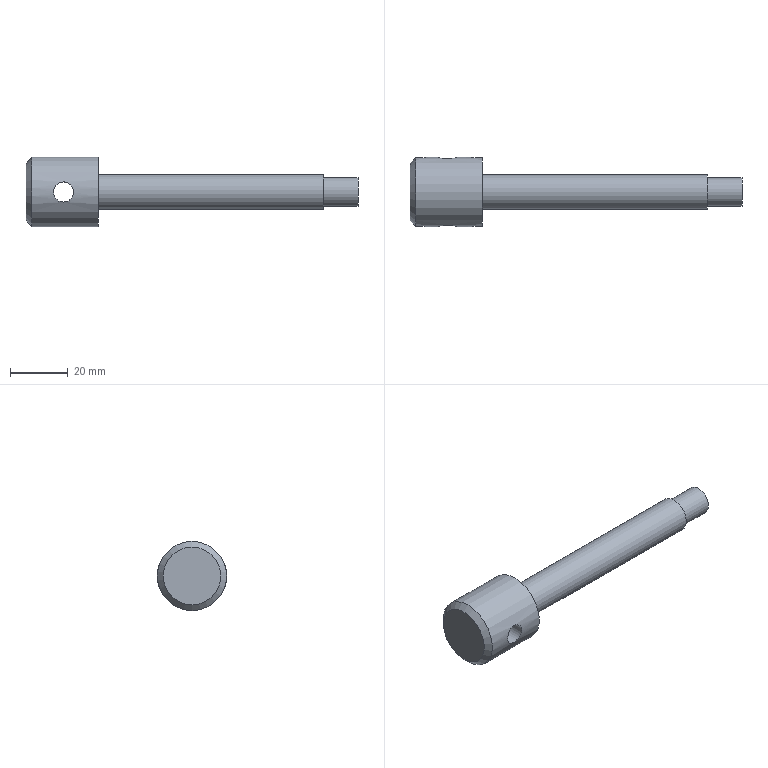Part | NX | features CYLINDER 3, CHAMFER 1, DATUM_CSYS 1, HOLE PACKAGE 1, POINT 1, SIMPLE HOLE 1, SYMBOLIC_THREAD 1 | 1 solid | 9 faces | box 115 x 24 x 24 mm | volume 19981 mm3 | plane 4 | cylinder 4 | cone 1 | commonest cylinder face diameters 7 x1 9.8 x1 12 x1 24 x1
STEP:
#1=CARTESIAN_POINT('',(-25.,0.,10.));
#2=VERTEX_POINT('',#1);
#3=CARTESIAN_POINT('',(-25.,0.,0.));
#4=DIRECTION('',(-1.,0.,0.));
#5=DIRECTION('',(0.,0.,1.));
#6=AXIS2_PLACEMENT_3D('',#3,#4,#5);
#7=CIRCLE('',#6,10.);
#8=EDGE_CURVE('',#2,#2,#7,.T.);
#9=ORIENTED_EDGE('',*,*,#8,.T.);
#10=EDGE_LOOP('',(#9));
#11=FACE_BOUND('',#10,.T.);
#12=CARTESIAN_POINT('',(-25.,0.,0.));
#13=DIRECTION('',(-1.,0.,0.));
#14=DIRECTION('',(0.,0.,1.));
#15=AXIS2_PLACEMENT_3D('',#12,#13,#14);
#16=PLANE('',#15);
#17=ADVANCED_FACE('',(#11),#16,.T.);
#18=CARTESIAN_POINT('',(0.,0.,-6.));
#19=VERTEX_POINT('',#18);
#20=CARTESIAN_POINT('',(0.,0.,0.));
#21=DIRECTION('',(1.,0.,0.));
#22=DIRECTION('',(0.,0.,-1.));
#23=AXIS2_PLACEMENT_3D('',#20,#21,#22);
#24=CIRCLE('',#23,6.);
#25=EDGE_CURVE('',#19,#19,#24,.T.);
#26=ORIENTED_EDGE('',*,*,#25,.F.);
#27=EDGE_LOOP('',(#26));
#28=FACE_BOUND('',#27,.T.);
#29=CARTESIAN_POINT('',(0.,0.,12.));
#30=VERTEX_POINT('',#29);
#31=CARTESIAN_POINT('',(0.,0.,0.));
#32=DIRECTION('',(-1.,0.,0.));
#33=DIRECTION('',(0.,0.,1.));
#34=AXIS2_PLACEMENT_3D('',#31,#32,#33);
#35=CIRCLE('',#34,12.);
#36=EDGE_CURVE('',#30,#30,#35,.T.);
#37=ORIENTED_EDGE('',*,*,#36,.F.);
#38=EDGE_LOOP('',(#37));
#39=FACE_BOUND('',#38,.T.);
#40=CARTESIAN_POINT('',(0.,0.,0.));
#41=DIRECTION('',(1.,0.,0.));
#42=DIRECTION('',(0.,0.,-1.));
#43=AXIS2_PLACEMENT_3D('',#40,#41,#42);
#44=PLANE('',#43);
#45=ADVANCED_FACE('',(#28,#39),#44,.T.);
#46=CARTESIAN_POINT('',(-23.,0.,12.));
#47=VERTEX_POINT('',#46);
#48=CARTESIAN_POINT('',(-23.,0.,0.));
#49=DIRECTION('',(-1.,0.,0.));
#50=DIRECTION('',(0.,0.,1.));
#51=AXIS2_PLACEMENT_3D('',#48,#49,#50);
#52=CIRCLE('',#51,12.);
#53=EDGE_CURVE('',#47,#47,#52,.F.);
#54=ORIENTED_EDGE('',*,*,#53,.T.);
#55=EDGE_LOOP('',(#54));
#56=FACE_BOUND('',#55,.T.);
#57=CARTESIAN_POINT('',(-12.,-11.478,3.5));
#58=VERTEX_POINT('',#57);
#59=CARTESIAN_POINT('',(-9.256,-11.745,2.741));
#60=CARTESIAN_POINT('',(-12.,-11.345,3.879));
#61=CARTESIAN_POINT('',(-14.743,-11.745,2.741));
#62=CARTESIAN_POINT('',(-15.879,-12.128,0.004281));
#63=CARTESIAN_POINT('',(-14.742,-11.745,-2.745));
#64=CARTESIAN_POINT('',(-12.002,-11.345,-3.878));
#65=CARTESIAN_POINT('',(-9.259,-11.744,-2.745));
#66=CARTESIAN_POINT('',(-8.121,-12.128,-0.0006967));
#67=CARTESIAN_POINT('',(-9.256,-11.745,2.741));
#68=CARTESIAN_POINT('',(-12.,-11.345,3.879));
#69=CARTESIAN_POINT('',(-14.743,-11.745,2.741));
#70=B_SPLINE_CURVE_WITH_KNOTS('',3,(#59,#60,#61,#62,#63,#64,#65,#66,#67,#68,#69),.UNSPECIFIED.,.T.,.F.,(1,1,1,1,1,1,1,1,1,1,1,1,1,1,1),(-0.008251,-0.005501,-0.00275,0.,0.00275,0.005501,0.008251,0.011,0.01375,0.0165,0.01925,0.022,0.02475,0.0275,0.03025),.UNSPECIFIED.);
#71=EDGE_CURVE('',#58,#58,#70,.T.);
#72=ORIENTED_EDGE('',*,*,#71,.F.);
#73=EDGE_LOOP('',(#72));
#74=FACE_BOUND('',#73,.T.);
#75=CARTESIAN_POINT('',(-12.,11.478,3.5));
#76=VERTEX_POINT('',#75);
#77=CARTESIAN_POINT('',(-14.744,11.745,2.741));
#78=CARTESIAN_POINT('',(-12.,11.345,3.879));
#79=CARTESIAN_POINT('',(-9.257,11.745,2.741));
#80=CARTESIAN_POINT('',(-8.121,12.128,0.004281));
#81=CARTESIAN_POINT('',(-9.258,11.745,-2.745));
#82=CARTESIAN_POINT('',(-11.998,11.345,-3.878));
#83=CARTESIAN_POINT('',(-14.741,11.744,-2.745));
#84=CARTESIAN_POINT('',(-15.879,12.128,-0.0006967));
#85=CARTESIAN_POINT('',(-14.744,11.745,2.741));
#86=CARTESIAN_POINT('',(-12.,11.345,3.879));
#87=CARTESIAN_POINT('',(-9.257,11.745,2.741));
#88=B_SPLINE_CURVE_WITH_KNOTS('',3,(#77,#78,#79,#80,#81,#82,#83,#84,#85,#86,#87),.UNSPECIFIED.,.T.,.F.,(1,1,1,1,1,1,1,1,1,1,1,1,1,1,1),(-0.008251,-0.005501,-0.00275,0.,0.00275,0.005501,0.008251,0.011,0.01375,0.0165,0.01925,0.022,0.02475,0.0275,0.03025),.UNSPECIFIED.);
#89=EDGE_CURVE('',#76,#76,#88,.T.);
#90=ORIENTED_EDGE('',*,*,#89,.F.);
#91=EDGE_LOOP('',(#90));
#92=FACE_BOUND('',#91,.T.);
#93=ORIENTED_EDGE('',*,*,#36,.T.);
#94=EDGE_LOOP('',(#93));
#95=FACE_BOUND('',#94,.T.);
#96=CARTESIAN_POINT('',(0.,0.,0.));
#97=DIRECTION('',(-1.,0.,0.));
#98=DIRECTION('',(0.,0.,1.));
#99=AXIS2_PLACEMENT_3D('',#96,#97,#98);
#100=CYLINDRICAL_SURFACE('',#99,12.);
#101=ADVANCED_FACE('',(#56,#74,#92,#95),#100,.T.);
#102=CARTESIAN_POINT('',(78.,0.,-4.9));
#103=VERTEX_POINT('',#102);
#104=CARTESIAN_POINT('',(78.,0.,0.));
#105=DIRECTION('',(1.,0.,0.));
#106=DIRECTION('',(0.,0.,-1.));
#107=AXIS2_PLACEMENT_3D('',#104,#105,#106);
#108=CIRCLE('',#107,4.9);
#109=EDGE_CURVE('',#103,#103,#108,.T.);
#110=ORIENTED_EDGE('',*,*,#109,.F.);
#111=EDGE_LOOP('',(#110));
#112=FACE_BOUND('',#111,.T.);
#113=CARTESIAN_POINT('',(78.,0.,-6.));
#114=VERTEX_POINT('',#113);
#115=CARTESIAN_POINT('',(78.,0.,0.));
#116=DIRECTION('',(-1.,0.,0.));
#117=DIRECTION('',(0.,0.,-1.));
#118=AXIS2_PLACEMENT_3D('',#115,#116,#117);
#119=CIRCLE('',#118,6.);
#120=EDGE_CURVE('',#114,#114,#119,.T.);
#121=ORIENTED_EDGE('',*,*,#120,.F.);
#122=EDGE_LOOP('',(#121));
#123=FACE_BOUND('',#122,.T.);
#124=CARTESIAN_POINT('',(78.,0.,0.));
#125=DIRECTION('',(1.,0.,0.));
#126=DIRECTION('',(0.,0.,-1.));
#127=AXIS2_PLACEMENT_3D('',#124,#125,#126);
#128=PLANE('',#127);
#129=ADVANCED_FACE('',(#112,#123),#128,.T.);
#130=ORIENTED_EDGE('',*,*,#120,.T.);
#131=EDGE_LOOP('',(#130));
#132=FACE_BOUND('',#131,.T.);
#133=ORIENTED_EDGE('',*,*,#25,.T.);
#134=EDGE_LOOP('',(#133));
#135=FACE_BOUND('',#134,.T.);
#136=CARTESIAN_POINT('',(0.,0.,0.));
#137=DIRECTION('',(1.,0.,0.));
#138=DIRECTION('',(0.,0.,-1.));
#139=AXIS2_PLACEMENT_3D('',#136,#137,#138);
#140=CYLINDRICAL_SURFACE('',#139,6.);
#141=ADVANCED_FACE('',(#132,#135),#140,.T.);
#142=CARTESIAN_POINT('',(90.,0.,-4.9));
#143=VERTEX_POINT('',#142);
#144=CARTESIAN_POINT('',(90.,0.,0.));
#145=DIRECTION('',(-1.,0.,0.));
#146=DIRECTION('',(0.,0.,-1.));
#147=AXIS2_PLACEMENT_3D('',#144,#145,#146);
#148=CIRCLE('',#147,4.9);
#149=EDGE_CURVE('',#143,#143,#148,.T.);
#150=ORIENTED_EDGE('',*,*,#149,.F.);
#151=EDGE_LOOP('',(#150));
#152=FACE_BOUND('',#151,.T.);
#153=CARTESIAN_POINT('',(90.,0.,0.));
#154=DIRECTION('',(1.,0.,0.));
#155=DIRECTION('',(0.,0.,-1.));
#156=AXIS2_PLACEMENT_3D('',#153,#154,#155);
#157=PLANE('',#156);
#158=ADVANCED_FACE('',(#152),#157,.T.);
#159=ORIENTED_EDGE('',*,*,#109,.T.);
#160=EDGE_LOOP('',(#159));
#161=FACE_BOUND('',#160,.T.);
#162=ORIENTED_EDGE('',*,*,#149,.T.);
#163=EDGE_LOOP('',(#162));
#164=FACE_BOUND('',#163,.T.);
#165=CARTESIAN_POINT('',(0.,0.,0.));
#166=DIRECTION('',(1.,0.,0.));
#167=DIRECTION('',(0.,0.,-1.));
#168=AXIS2_PLACEMENT_3D('',#165,#166,#167);
#169=CYLINDRICAL_SURFACE('',#168,4.9);
#170=ADVANCED_FACE('',(#161,#164),#169,.T.);
#171=ORIENTED_EDGE('',*,*,#71,.T.);
#172=EDGE_LOOP('',(#171));
#173=FACE_BOUND('',#172,.T.);
#174=ORIENTED_EDGE('',*,*,#89,.T.);
#175=EDGE_LOOP('',(#174));
#176=FACE_BOUND('',#175,.T.);
#177=CARTESIAN_POINT('',(-12.,-12.,0.));
#178=DIRECTION('',(0.,1.,0.));
#179=DIRECTION('',(0.,0.,1.));
#180=AXIS2_PLACEMENT_3D('',#177,#178,#179);
#181=CYLINDRICAL_SURFACE('',#180,3.5);
#182=ADVANCED_FACE('',(#173,#176),#181,.F.);
#183=ORIENTED_EDGE('',*,*,#8,.F.);
#184=EDGE_LOOP('',(#183));
#185=FACE_BOUND('',#184,.T.);
#186=ORIENTED_EDGE('',*,*,#53,.F.);
#187=EDGE_LOOP('',(#186));
#188=FACE_BOUND('',#187,.T.);
#189=CARTESIAN_POINT('',(-23.,0.,0.));
#190=DIRECTION('',(1.,0.,0.));
#191=DIRECTION('',(0.,0.,-1.));
#192=AXIS2_PLACEMENT_3D('',#189,#190,#191);
#193=CONICAL_SURFACE('',#192,12.,0.7854);
#194=ADVANCED_FACE('',(#185,#188),#193,.T.);
#195=CLOSED_SHELL('',(#17,#45,#101,#129,#141,#158,#170,#182,#194));
#196=MANIFOLD_SOLID_BREP('',#195);
#197=(LENGTH_UNIT()NAMED_UNIT(*)SI_UNIT(.MILLI.,.METRE.));
#198=UNCERTAINTY_MEASURE_WITH_UNIT(LENGTH_MEASURE(0.0508),#197,'','');
#199=(NAMED_UNIT(*)PLANE_ANGLE_UNIT()SI_UNIT($,.RADIAN.));
#200=(NAMED_UNIT(*)SI_UNIT($,.STERADIAN.)SOLID_ANGLE_UNIT());
#201=(GEOMETRIC_REPRESENTATION_CONTEXT(3)GLOBAL_UNCERTAINTY_ASSIGNED_CONTEXT((#198))GLOBAL_UNIT_ASSIGNED_CONTEXT((#197,#199,#200))REPRESENTATION_CONTEXT('',''));
#202=ADVANCED_BREP_SHAPE_REPRESENTATION('',(#196),#201);